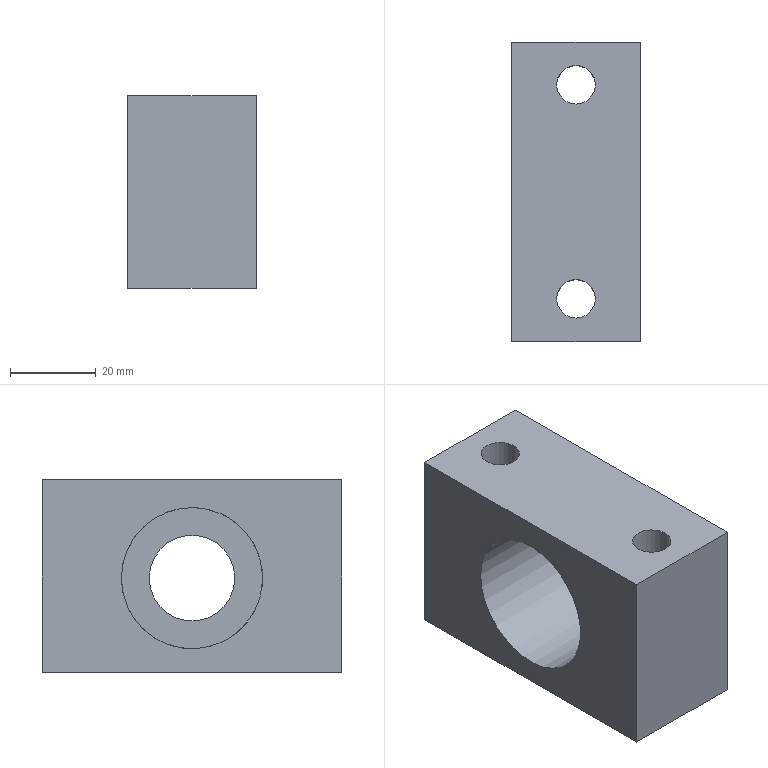Part | NX | features solid 2 | 1 solid | 15 faces | box 30 x 70 x 45 mm | volume 60223 mm3 | plane 9 | cylinder 6 | commonest cylinder face diameters 9 x2 14 x2 20 x1 33 x1
STEP:
#1=CARTESIAN_POINT('',(956.701,86.3,211.));
#2=VERTEX_POINT('',#1);
#3=CARTESIAN_POINT('',(956.701,90.8,211.));
#4=DIRECTION('',(0.,0.,1.));
#5=DIRECTION('',(0.,-1.,0.));
#6=AXIS2_PLACEMENT_3D('',#3,#4,#5);
#7=CIRCLE('',#6,4.5);
#8=EDGE_CURVE('',#2,#2,#7,.T.);
#9=ORIENTED_EDGE('',*,*,#8,.F.);
#10=EDGE_LOOP('',(#9));
#11=FACE_BOUND('',#10,.T.);
#12=CARTESIAN_POINT('',(956.701,136.3,211.));
#13=VERTEX_POINT('',#12);
#14=CARTESIAN_POINT('',(956.701,140.8,211.));
#15=DIRECTION('',(0.,0.,1.));
#16=DIRECTION('',(0.,-1.,0.));
#17=AXIS2_PLACEMENT_3D('',#14,#15,#16);
#18=CIRCLE('',#17,4.5);
#19=EDGE_CURVE('',#13,#13,#18,.T.);
#20=ORIENTED_EDGE('',*,*,#19,.F.);
#21=EDGE_LOOP('',(#20));
#22=FACE_BOUND('',#21,.T.);
#23=CARTESIAN_POINT('',(941.701,80.8,211.));
#24=VERTEX_POINT('',#23);
#25=CARTESIAN_POINT('',(941.701,150.8,211.));
#26=VERTEX_POINT('',#25);
#27=CARTESIAN_POINT('',(941.701,85.8,211.));
#28=DIRECTION('',(0.,1.,0.));
#29=VECTOR('',#28,1000.);
#30=LINE('',#27,#29);
#31=EDGE_CURVE('',#24,#26,#30,.T.);
#32=ORIENTED_EDGE('',*,*,#31,.F.);
#33=CARTESIAN_POINT('',(971.701,80.8,211.));
#34=VERTEX_POINT('',#33);
#35=CARTESIAN_POINT('',(991.701,80.8,211.));
#36=DIRECTION('',(-1.,0.,0.));
#37=VECTOR('',#36,1000.);
#38=LINE('',#35,#37);
#39=EDGE_CURVE('',#34,#24,#38,.T.);
#40=ORIENTED_EDGE('',*,*,#39,.F.);
#41=CARTESIAN_POINT('',(971.701,150.8,211.));
#42=VERTEX_POINT('',#41);
#43=CARTESIAN_POINT('',(971.701,85.8,211.));
#44=DIRECTION('',(0.,1.,0.));
#45=VECTOR('',#44,1000.);
#46=LINE('',#43,#45);
#47=EDGE_CURVE('',#34,#42,#46,.T.);
#48=ORIENTED_EDGE('',*,*,#47,.T.);
#49=CARTESIAN_POINT('',(991.701,150.8,211.));
#50=DIRECTION('',(-1.,0.,0.));
#51=VECTOR('',#50,1000.);
#52=LINE('',#49,#51);
#53=EDGE_CURVE('',#42,#26,#52,.T.);
#54=ORIENTED_EDGE('',*,*,#53,.T.);
#55=EDGE_LOOP('',(#32,#40,#48,#54));
#56=FACE_BOUND('',#55,.T.);
#57=CARTESIAN_POINT('',(991.701,85.8,211.));
#58=DIRECTION('',(0.,0.,-1.));
#59=DIRECTION('',(0.,-1.,0.));
#60=AXIS2_PLACEMENT_3D('',#57,#58,#59);
#61=PLANE('',#60);
#62=ADVANCED_FACE('',(#11,#22,#56),#61,.F.);
#63=CARTESIAN_POINT('',(941.701,150.8,166.));
#64=VERTEX_POINT('',#63);
#65=CARTESIAN_POINT('',(941.701,150.8,166.));
#66=DIRECTION('',(0.,0.,1.));
#67=VECTOR('',#66,1000.);
#68=LINE('',#65,#67);
#69=EDGE_CURVE('',#64,#26,#68,.T.);
#70=ORIENTED_EDGE('',*,*,#69,.T.);
#71=ORIENTED_EDGE('',*,*,#53,.F.);
#72=CARTESIAN_POINT('',(971.701,150.8,166.));
#73=VERTEX_POINT('',#72);
#74=CARTESIAN_POINT('',(971.701,150.8,166.));
#75=DIRECTION('',(0.,0.,1.));
#76=VECTOR('',#75,1000.);
#77=LINE('',#74,#76);
#78=EDGE_CURVE('',#73,#42,#77,.T.);
#79=ORIENTED_EDGE('',*,*,#78,.F.);
#80=CARTESIAN_POINT('',(991.701,150.8,166.));
#81=DIRECTION('',(-1.,0.,0.));
#82=VECTOR('',#81,1000.);
#83=LINE('',#80,#82);
#84=EDGE_CURVE('',#73,#64,#83,.T.);
#85=ORIENTED_EDGE('',*,*,#84,.T.);
#86=EDGE_LOOP('',(#70,#71,#79,#85));
#87=FACE_BOUND('',#86,.T.);
#88=CARTESIAN_POINT('',(991.701,150.8,166.));
#89=DIRECTION('',(0.,1.,0.));
#90=DIRECTION('',(0.,0.,-1.));
#91=AXIS2_PLACEMENT_3D('',#88,#89,#90);
#92=PLANE('',#91);
#93=ADVANCED_FACE('',(#87),#92,.T.);
#94=CARTESIAN_POINT('',(956.701,97.8,166.));
#95=VERTEX_POINT('',#94);
#96=CARTESIAN_POINT('',(956.701,90.8,166.));
#97=DIRECTION('',(0.,0.,-1.));
#98=DIRECTION('',(0.,1.,0.));
#99=AXIS2_PLACEMENT_3D('',#96,#97,#98);
#100=CIRCLE('',#99,7.);
#101=EDGE_CURVE('',#95,#95,#100,.T.);
#102=ORIENTED_EDGE('',*,*,#101,.F.);
#103=EDGE_LOOP('',(#102));
#104=FACE_BOUND('',#103,.T.);
#105=CARTESIAN_POINT('',(956.701,147.8,166.));
#106=VERTEX_POINT('',#105);
#107=CARTESIAN_POINT('',(956.701,140.8,166.));
#108=DIRECTION('',(0.,0.,-1.));
#109=DIRECTION('',(0.,1.,0.));
#110=AXIS2_PLACEMENT_3D('',#107,#108,#109);
#111=CIRCLE('',#110,7.);
#112=EDGE_CURVE('',#106,#106,#111,.T.);
#113=ORIENTED_EDGE('',*,*,#112,.F.);
#114=EDGE_LOOP('',(#113));
#115=FACE_BOUND('',#114,.T.);
#116=CARTESIAN_POINT('',(941.701,80.8,166.));
#117=VERTEX_POINT('',#116);
#118=CARTESIAN_POINT('',(941.701,85.8,166.));
#119=DIRECTION('',(0.,1.,0.));
#120=VECTOR('',#119,1000.);
#121=LINE('',#118,#120);
#122=EDGE_CURVE('',#117,#64,#121,.T.);
#123=ORIENTED_EDGE('',*,*,#122,.T.);
#124=ORIENTED_EDGE('',*,*,#84,.F.);
#125=CARTESIAN_POINT('',(971.701,80.8,166.));
#126=VERTEX_POINT('',#125);
#127=CARTESIAN_POINT('',(971.701,85.8,166.));
#128=DIRECTION('',(0.,1.,0.));
#129=VECTOR('',#128,1000.);
#130=LINE('',#127,#129);
#131=EDGE_CURVE('',#126,#73,#130,.T.);
#132=ORIENTED_EDGE('',*,*,#131,.F.);
#133=CARTESIAN_POINT('',(991.701,80.8,166.));
#134=DIRECTION('',(-1.,0.,0.));
#135=VECTOR('',#134,1000.);
#136=LINE('',#133,#135);
#137=EDGE_CURVE('',#126,#117,#136,.T.);
#138=ORIENTED_EDGE('',*,*,#137,.T.);
#139=EDGE_LOOP('',(#123,#124,#132,#138));
#140=FACE_BOUND('',#139,.T.);
#141=CARTESIAN_POINT('',(991.701,85.8,166.));
#142=DIRECTION('',(0.,0.,-1.));
#143=DIRECTION('',(0.,-1.,0.));
#144=AXIS2_PLACEMENT_3D('',#141,#142,#143);
#145=PLANE('',#144);
#146=ADVANCED_FACE('',(#104,#115,#140),#145,.T.);
#147=CARTESIAN_POINT('',(941.701,80.8,166.));
#148=DIRECTION('',(0.,0.,1.));
#149=VECTOR('',#148,1000.);
#150=LINE('',#147,#149);
#151=EDGE_CURVE('',#117,#24,#150,.T.);
#152=ORIENTED_EDGE('',*,*,#151,.F.);
#153=ORIENTED_EDGE('',*,*,#137,.F.);
#154=CARTESIAN_POINT('',(971.701,80.8,166.));
#155=DIRECTION('',(0.,0.,1.));
#156=VECTOR('',#155,1000.);
#157=LINE('',#154,#156);
#158=EDGE_CURVE('',#126,#34,#157,.T.);
#159=ORIENTED_EDGE('',*,*,#158,.T.);
#160=ORIENTED_EDGE('',*,*,#39,.T.);
#161=EDGE_LOOP('',(#152,#153,#159,#160));
#162=FACE_BOUND('',#161,.T.);
#163=CARTESIAN_POINT('',(991.701,80.8,166.));
#164=DIRECTION('',(0.,1.,0.));
#165=DIRECTION('',(0.,0.,-1.));
#166=AXIS2_PLACEMENT_3D('',#163,#164,#165);
#167=PLANE('',#166);
#168=ADVANCED_FACE('',(#162),#167,.F.);
#169=CARTESIAN_POINT('',(971.701,125.8,188.));
#170=VERTEX_POINT('',#169);
#171=CARTESIAN_POINT('',(971.701,115.8,188.));
#172=DIRECTION('',(1.,0.,0.));
#173=DIRECTION('',(0.,1.,0.));
#174=AXIS2_PLACEMENT_3D('',#171,#172,#173);
#175=CIRCLE('',#174,10.);
#176=EDGE_CURVE('',#170,#170,#175,.T.);
#177=ORIENTED_EDGE('',*,*,#176,.F.);
#178=EDGE_LOOP('',(#177));
#179=FACE_BOUND('',#178,.T.);
#180=ORIENTED_EDGE('',*,*,#47,.F.);
#181=ORIENTED_EDGE('',*,*,#158,.F.);
#182=ORIENTED_EDGE('',*,*,#131,.T.);
#183=ORIENTED_EDGE('',*,*,#78,.T.);
#184=EDGE_LOOP('',(#180,#181,#182,#183));
#185=FACE_BOUND('',#184,.T.);
#186=CARTESIAN_POINT('',(971.701,85.8,166.));
#187=DIRECTION('',(-1.,0.,0.));
#188=DIRECTION('',(0.,0.,1.));
#189=AXIS2_PLACEMENT_3D('',#186,#187,#188);
#190=PLANE('',#189);
#191=ADVANCED_FACE('',(#179,#185),#190,.F.);
#192=CARTESIAN_POINT('',(941.701,132.3,188.));
#193=VERTEX_POINT('',#192);
#194=CARTESIAN_POINT('',(941.701,115.8,188.));
#195=DIRECTION('',(1.,0.,0.));
#196=DIRECTION('',(0.,1.,0.));
#197=AXIS2_PLACEMENT_3D('',#194,#195,#196);
#198=CIRCLE('',#197,16.5);
#199=EDGE_CURVE('',#193,#193,#198,.T.);
#200=ORIENTED_EDGE('',*,*,#199,.T.);
#201=EDGE_LOOP('',(#200));
#202=FACE_BOUND('',#201,.T.);
#203=ORIENTED_EDGE('',*,*,#31,.T.);
#204=ORIENTED_EDGE('',*,*,#69,.F.);
#205=ORIENTED_EDGE('',*,*,#122,.F.);
#206=ORIENTED_EDGE('',*,*,#151,.T.);
#207=EDGE_LOOP('',(#203,#204,#205,#206));
#208=FACE_BOUND('',#207,.T.);
#209=CARTESIAN_POINT('',(941.701,85.8,166.));
#210=DIRECTION('',(-1.,0.,0.));
#211=DIRECTION('',(0.,0.,1.));
#212=AXIS2_PLACEMENT_3D('',#209,#210,#211);
#213=PLANE('',#212);
#214=ADVANCED_FACE('',(#202,#208),#213,.T.);
#215=CARTESIAN_POINT('',(956.701,145.3,191.));
#216=VERTEX_POINT('',#215);
#217=CARTESIAN_POINT('',(956.701,140.8,191.));
#218=DIRECTION('',(0.,0.,-1.));
#219=DIRECTION('',(0.,1.,0.));
#220=AXIS2_PLACEMENT_3D('',#217,#218,#219);
#221=CIRCLE('',#220,4.5);
#222=EDGE_CURVE('',#216,#216,#221,.T.);
#223=ORIENTED_EDGE('',*,*,#222,.T.);
#224=EDGE_LOOP('',(#223));
#225=FACE_BOUND('',#224,.T.);
#226=ORIENTED_EDGE('',*,*,#19,.T.);
#227=EDGE_LOOP('',(#226));
#228=FACE_BOUND('',#227,.T.);
#229=CARTESIAN_POINT('',(956.701,140.8,216.));
#230=DIRECTION('',(0.,0.,1.));
#231=DIRECTION('',(0.,1.,0.));
#232=AXIS2_PLACEMENT_3D('',#229,#230,#231);
#233=CYLINDRICAL_SURFACE('',#232,4.5);
#234=ADVANCED_FACE('',(#225,#228),#233,.F.);
#235=ORIENTED_EDGE('',*,*,#222,.F.);
#236=EDGE_LOOP('',(#235));
#237=FACE_BOUND('',#236,.T.);
#238=CARTESIAN_POINT('',(956.701,147.8,191.));
#239=VERTEX_POINT('',#238);
#240=CARTESIAN_POINT('',(956.701,140.8,191.));
#241=DIRECTION('',(0.,0.,-1.));
#242=DIRECTION('',(0.,1.,0.));
#243=AXIS2_PLACEMENT_3D('',#240,#241,#242);
#244=CIRCLE('',#243,7.);
#245=EDGE_CURVE('',#239,#239,#244,.T.);
#246=ORIENTED_EDGE('',*,*,#245,.T.);
#247=EDGE_LOOP('',(#246));
#248=FACE_BOUND('',#247,.T.);
#249=CARTESIAN_POINT('',(956.701,140.8,191.));
#250=DIRECTION('',(0.,0.,1.));
#251=DIRECTION('',(0.,1.,0.));
#252=AXIS2_PLACEMENT_3D('',#249,#250,#251);
#253=PLANE('',#252);
#254=ADVANCED_FACE('',(#237,#248),#253,.F.);
#255=ORIENTED_EDGE('',*,*,#245,.F.);
#256=EDGE_LOOP('',(#255));
#257=FACE_BOUND('',#256,.T.);
#258=ORIENTED_EDGE('',*,*,#112,.T.);
#259=EDGE_LOOP('',(#258));
#260=FACE_BOUND('',#259,.T.);
#261=CARTESIAN_POINT('',(956.701,140.8,166.));
#262=DIRECTION('',(0.,0.,1.));
#263=DIRECTION('',(0.,1.,0.));
#264=AXIS2_PLACEMENT_3D('',#261,#262,#263);
#265=CYLINDRICAL_SURFACE('',#264,7.);
#266=ADVANCED_FACE('',(#257,#260),#265,.F.);
#267=CARTESIAN_POINT('',(956.701,95.3,191.));
#268=VERTEX_POINT('',#267);
#269=CARTESIAN_POINT('',(956.701,90.8,191.));
#270=DIRECTION('',(0.,0.,-1.));
#271=DIRECTION('',(0.,1.,0.));
#272=AXIS2_PLACEMENT_3D('',#269,#270,#271);
#273=CIRCLE('',#272,4.5);
#274=EDGE_CURVE('',#268,#268,#273,.T.);
#275=ORIENTED_EDGE('',*,*,#274,.T.);
#276=EDGE_LOOP('',(#275));
#277=FACE_BOUND('',#276,.T.);
#278=ORIENTED_EDGE('',*,*,#8,.T.);
#279=EDGE_LOOP('',(#278));
#280=FACE_BOUND('',#279,.T.);
#281=CARTESIAN_POINT('',(956.701,90.8,216.));
#282=DIRECTION('',(0.,0.,1.));
#283=DIRECTION('',(0.,1.,0.));
#284=AXIS2_PLACEMENT_3D('',#281,#282,#283);
#285=CYLINDRICAL_SURFACE('',#284,4.5);
#286=ADVANCED_FACE('',(#277,#280),#285,.F.);
#287=ORIENTED_EDGE('',*,*,#274,.F.);
#288=EDGE_LOOP('',(#287));
#289=FACE_BOUND('',#288,.T.);
#290=CARTESIAN_POINT('',(956.701,97.8,191.));
#291=VERTEX_POINT('',#290);
#292=CARTESIAN_POINT('',(956.701,90.8,191.));
#293=DIRECTION('',(0.,0.,-1.));
#294=DIRECTION('',(0.,1.,0.));
#295=AXIS2_PLACEMENT_3D('',#292,#293,#294);
#296=CIRCLE('',#295,7.);
#297=EDGE_CURVE('',#291,#291,#296,.T.);
#298=ORIENTED_EDGE('',*,*,#297,.T.);
#299=EDGE_LOOP('',(#298));
#300=FACE_BOUND('',#299,.T.);
#301=CARTESIAN_POINT('',(956.701,90.8,191.));
#302=DIRECTION('',(0.,0.,1.));
#303=DIRECTION('',(0.,1.,0.));
#304=AXIS2_PLACEMENT_3D('',#301,#302,#303);
#305=PLANE('',#304);
#306=ADVANCED_FACE('',(#289,#300),#305,.F.);
#307=ORIENTED_EDGE('',*,*,#297,.F.);
#308=EDGE_LOOP('',(#307));
#309=FACE_BOUND('',#308,.T.);
#310=ORIENTED_EDGE('',*,*,#101,.T.);
#311=EDGE_LOOP('',(#310));
#312=FACE_BOUND('',#311,.T.);
#313=CARTESIAN_POINT('',(956.701,90.8,166.));
#314=DIRECTION('',(0.,0.,1.));
#315=DIRECTION('',(0.,1.,0.));
#316=AXIS2_PLACEMENT_3D('',#313,#314,#315);
#317=CYLINDRICAL_SURFACE('',#316,7.);
#318=ADVANCED_FACE('',(#309,#312),#317,.F.);
#319=CARTESIAN_POINT('',(968.701,105.8,188.));
#320=VERTEX_POINT('',#319);
#321=CARTESIAN_POINT('',(968.701,115.8,188.));
#322=DIRECTION('',(-1.,0.,0.));
#323=DIRECTION('',(0.,-1.,0.));
#324=AXIS2_PLACEMENT_3D('',#321,#322,#323);
#325=CIRCLE('',#324,10.);
#326=EDGE_CURVE('',#320,#320,#325,.F.);
#327=ORIENTED_EDGE('',*,*,#326,.F.);
#328=EDGE_LOOP('',(#327));
#329=FACE_BOUND('',#328,.T.);
#330=ORIENTED_EDGE('',*,*,#176,.T.);
#331=EDGE_LOOP('',(#330));
#332=FACE_BOUND('',#331,.T.);
#333=CARTESIAN_POINT('',(1052.701,115.8,188.));
#334=DIRECTION('',(1.,0.,0.));
#335=DIRECTION('',(0.,0.,-1.));
#336=AXIS2_PLACEMENT_3D('',#333,#334,#335);
#337=CYLINDRICAL_SURFACE('',#336,10.);
#338=ADVANCED_FACE('',(#329,#332),#337,.F.);
#339=ORIENTED_EDGE('',*,*,#326,.T.);
#340=EDGE_LOOP('',(#339));
#341=FACE_BOUND('',#340,.T.);
#342=CARTESIAN_POINT('',(968.701,99.3,188.));
#343=VERTEX_POINT('',#342);
#344=CARTESIAN_POINT('',(968.701,115.8,188.));
#345=DIRECTION('',(-1.,0.,0.));
#346=DIRECTION('',(0.,-1.,0.));
#347=AXIS2_PLACEMENT_3D('',#344,#345,#346);
#348=CIRCLE('',#347,16.5);
#349=EDGE_CURVE('',#343,#343,#348,.T.);
#350=ORIENTED_EDGE('',*,*,#349,.T.);
#351=EDGE_LOOP('',(#350));
#352=FACE_BOUND('',#351,.T.);
#353=CARTESIAN_POINT('',(968.701,115.8,188.));
#354=DIRECTION('',(1.,0.,0.));
#355=DIRECTION('',(0.,0.,-1.));
#356=AXIS2_PLACEMENT_3D('',#353,#354,#355);
#357=PLANE('',#356);
#358=ADVANCED_FACE('',(#341,#352),#357,.F.);
#359=ORIENTED_EDGE('',*,*,#199,.F.);
#360=EDGE_LOOP('',(#359));
#361=FACE_BOUND('',#360,.T.);
#362=ORIENTED_EDGE('',*,*,#349,.F.);
#363=EDGE_LOOP('',(#362));
#364=FACE_BOUND('',#363,.T.);
#365=CARTESIAN_POINT('',(880.701,115.8,188.));
#366=DIRECTION('',(1.,0.,0.));
#367=DIRECTION('',(0.,0.,-1.));
#368=AXIS2_PLACEMENT_3D('',#365,#366,#367);
#369=CYLINDRICAL_SURFACE('',#368,16.5);
#370=ADVANCED_FACE('',(#361,#364),#369,.F.);
#371=CLOSED_SHELL('',(#62,#93,#146,#168,#191,#214,#234,#254,#266,#286,#306,#318,#338,#358,#370));
#372=MANIFOLD_SOLID_BREP('',#371);
#373=(LENGTH_UNIT()NAMED_UNIT(*)SI_UNIT(.MILLI.,.METRE.));
#374=UNCERTAINTY_MEASURE_WITH_UNIT(LENGTH_MEASURE(0.00001),#373,'','');
#375=(NAMED_UNIT(*)PLANE_ANGLE_UNIT()SI_UNIT($,.RADIAN.));
#376=(NAMED_UNIT(*)SI_UNIT($,.STERADIAN.)SOLID_ANGLE_UNIT());
#377=(GEOMETRIC_REPRESENTATION_CONTEXT(3)GLOBAL_UNCERTAINTY_ASSIGNED_CONTEXT((#374))GLOBAL_UNIT_ASSIGNED_CONTEXT((#373,#375,#376))REPRESENTATION_CONTEXT('',''));
#378=ADVANCED_BREP_SHAPE_REPRESENTATION('',(#372),#377);